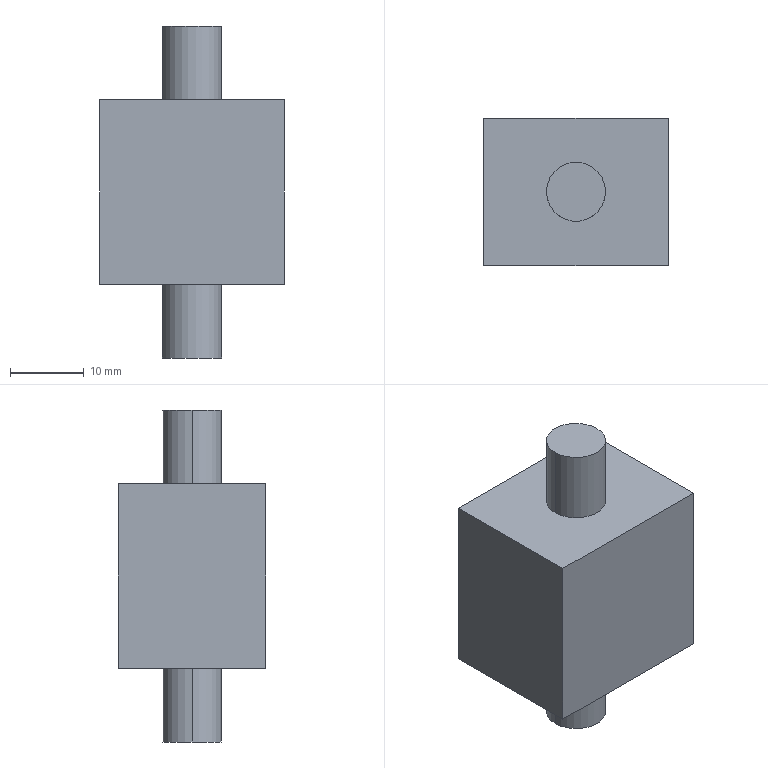Part | SolidWorks | features Extrusion 1, ICE 1, MirrorPattern 1 | 1 solid | 12 faces | box 25 x 20 x 45 mm | volume 13505 mm3 | plane 8 | cylinder 4 | commonest cylinder face diameters 8 x4
STEP:
#1=CARTESIAN_POINT('',(4.,10.,-22.5));
#2=VERTEX_POINT('',#1);
#3=CARTESIAN_POINT('',(-4.,10.,-22.5));
#4=VERTEX_POINT('',#3);
#5=CARTESIAN_POINT('',(0.,10.,-22.5));
#6=DIRECTION('',(0.,0.,1.));
#7=DIRECTION('',(1.,0.,0.));
#8=AXIS2_PLACEMENT_3D('',#5,#6,#7);
#9=CIRCLE('',#8,4.);
#10=EDGE_CURVE('',#2,#4,#9,.T.);
#11=ORIENTED_EDGE('',*,*,#10,.T.);
#12=CARTESIAN_POINT('',(-4.,10.,-12.5));
#13=VERTEX_POINT('',#12);
#14=CARTESIAN_POINT('',(-4.,10.,-22.5));
#15=DIRECTION('',(0.,0.,1.));
#16=VECTOR('',#15,1000.);
#17=LINE('',#14,#16);
#18=EDGE_CURVE('',#4,#13,#17,.T.);
#19=ORIENTED_EDGE('',*,*,#18,.T.);
#20=CARTESIAN_POINT('',(4.,10.,-12.5));
#21=VERTEX_POINT('',#20);
#22=CARTESIAN_POINT('',(0.,10.,-12.5));
#23=DIRECTION('',(0.,0.,1.));
#24=DIRECTION('',(1.,0.,0.));
#25=AXIS2_PLACEMENT_3D('',#22,#23,#24);
#26=CIRCLE('',#25,4.);
#27=EDGE_CURVE('',#21,#13,#26,.T.);
#28=ORIENTED_EDGE('',*,*,#27,.F.);
#29=CARTESIAN_POINT('',(4.,10.,-22.5));
#30=DIRECTION('',(0.,0.,1.));
#31=VECTOR('',#30,1000.);
#32=LINE('',#29,#31);
#33=EDGE_CURVE('',#2,#21,#32,.T.);
#34=ORIENTED_EDGE('',*,*,#33,.F.);
#35=EDGE_LOOP('',(#11,#19,#28,#34));
#36=FACE_OUTER_BOUND('',#35,.T.);
#37=CARTESIAN_POINT('',(0.,10.,-22.5));
#38=DIRECTION('',(0.,0.,1.));
#39=DIRECTION('',(1.,0.,0.));
#40=AXIS2_PLACEMENT_3D('',#37,#38,#39);
#41=CYLINDRICAL_SURFACE('',#40,4.);
#42=ADVANCED_FACE('',(#36),#41,.T.);
#43=CARTESIAN_POINT('',(4.,10.,22.5));
#44=VERTEX_POINT('',#43);
#45=CARTESIAN_POINT('',(-4.,10.,22.5));
#46=VERTEX_POINT('',#45);
#47=CARTESIAN_POINT('',(0.,10.,22.5));
#48=DIRECTION('',(0.,0.,1.));
#49=DIRECTION('',(1.,0.,0.));
#50=AXIS2_PLACEMENT_3D('',#47,#48,#49);
#51=CIRCLE('',#50,4.);
#52=EDGE_CURVE('',#44,#46,#51,.T.);
#53=ORIENTED_EDGE('',*,*,#52,.F.);
#54=CARTESIAN_POINT('',(4.,10.,12.5));
#55=VERTEX_POINT('',#54);
#56=CARTESIAN_POINT('',(4.,10.,22.5));
#57=DIRECTION('',(0.,0.,-1.));
#58=VECTOR('',#57,1000.);
#59=LINE('',#56,#58);
#60=EDGE_CURVE('',#44,#55,#59,.T.);
#61=ORIENTED_EDGE('',*,*,#60,.T.);
#62=CARTESIAN_POINT('',(-4.,10.,12.5));
#63=VERTEX_POINT('',#62);
#64=CARTESIAN_POINT('',(0.,10.,12.5));
#65=DIRECTION('',(0.,0.,1.));
#66=DIRECTION('',(1.,0.,0.));
#67=AXIS2_PLACEMENT_3D('',#64,#65,#66);
#68=CIRCLE('',#67,4.);
#69=EDGE_CURVE('',#55,#63,#68,.T.);
#70=ORIENTED_EDGE('',*,*,#69,.T.);
#71=CARTESIAN_POINT('',(-4.,10.,22.5));
#72=DIRECTION('',(0.,0.,-1.));
#73=VECTOR('',#72,1000.);
#74=LINE('',#71,#73);
#75=EDGE_CURVE('',#46,#63,#74,.T.);
#76=ORIENTED_EDGE('',*,*,#75,.F.);
#77=EDGE_LOOP('',(#53,#61,#70,#76));
#78=FACE_OUTER_BOUND('',#77,.T.);
#79=CARTESIAN_POINT('',(0.,10.,22.5));
#80=DIRECTION('',(0.,0.,-1.));
#81=DIRECTION('',(-1.,0.,0.));
#82=AXIS2_PLACEMENT_3D('',#79,#80,#81);
#83=CYLINDRICAL_SURFACE('',#82,4.);
#84=ADVANCED_FACE('',(#78),#83,.T.);
#85=CARTESIAN_POINT('',(12.5,0.,12.5));
#86=VERTEX_POINT('',#85);
#87=CARTESIAN_POINT('',(12.5,0.,-12.5));
#88=VERTEX_POINT('',#87);
#89=CARTESIAN_POINT('',(12.5,0.,12.5));
#90=DIRECTION('',(0.,0.,-1.));
#91=VECTOR('',#90,1000.);
#92=LINE('',#89,#91);
#93=EDGE_CURVE('',#86,#88,#92,.T.);
#94=ORIENTED_EDGE('',*,*,#93,.T.);
#95=CARTESIAN_POINT('',(12.5,20.,-12.5));
#96=VERTEX_POINT('',#95);
#97=CARTESIAN_POINT('',(12.5,20.,-12.5));
#98=DIRECTION('',(0.,-1.,0.));
#99=VECTOR('',#98,1000.);
#100=LINE('',#97,#99);
#101=EDGE_CURVE('',#96,#88,#100,.T.);
#102=ORIENTED_EDGE('',*,*,#101,.F.);
#103=CARTESIAN_POINT('',(12.5,20.,12.5));
#104=VERTEX_POINT('',#103);
#105=CARTESIAN_POINT('',(12.5,20.,12.5));
#106=DIRECTION('',(0.,0.,-1.));
#107=VECTOR('',#106,1000.);
#108=LINE('',#105,#107);
#109=EDGE_CURVE('',#104,#96,#108,.T.);
#110=ORIENTED_EDGE('',*,*,#109,.F.);
#111=CARTESIAN_POINT('',(12.5,20.,12.5));
#112=DIRECTION('',(0.,-1.,0.));
#113=VECTOR('',#112,1000.);
#114=LINE('',#111,#113);
#115=EDGE_CURVE('',#104,#86,#114,.T.);
#116=ORIENTED_EDGE('',*,*,#115,.T.);
#117=EDGE_LOOP('',(#94,#102,#110,#116));
#118=FACE_OUTER_BOUND('',#117,.T.);
#119=CARTESIAN_POINT('',(12.5,20.,12.5));
#120=DIRECTION('',(-1.,0.,0.));
#121=DIRECTION('',(0.,0.,1.));
#122=AXIS2_PLACEMENT_3D('',#119,#120,#121);
#123=PLANE('',#122);
#124=ADVANCED_FACE('',(#118),#123,.F.);
#125=ORIENTED_EDGE('',*,*,#27,.T.);
#126=CARTESIAN_POINT('',(0.,10.,-12.5));
#127=DIRECTION('',(0.,0.,1.));
#128=DIRECTION('',(1.,0.,0.));
#129=AXIS2_PLACEMENT_3D('',#126,#127,#128);
#130=CIRCLE('',#129,4.);
#131=EDGE_CURVE('',#13,#21,#130,.T.);
#132=ORIENTED_EDGE('',*,*,#131,.T.);
#133=EDGE_LOOP('',(#125,#132));
#134=FACE_BOUND('',#133,.T.);
#135=CARTESIAN_POINT('',(-12.5,0.,-12.5));
#136=VERTEX_POINT('',#135);
#137=CARTESIAN_POINT('',(-12.5,0.,-12.5));
#138=DIRECTION('',(-1.,0.,0.));
#139=VECTOR('',#138,1000.);
#140=LINE('',#137,#139);
#141=EDGE_CURVE('',#88,#136,#140,.T.);
#142=ORIENTED_EDGE('',*,*,#141,.T.);
#143=CARTESIAN_POINT('',(-12.5,20.,-12.5));
#144=VERTEX_POINT('',#143);
#145=CARTESIAN_POINT('',(-12.5,20.,-12.5));
#146=DIRECTION('',(0.,-1.,0.));
#147=VECTOR('',#146,1000.);
#148=LINE('',#145,#147);
#149=EDGE_CURVE('',#144,#136,#148,.T.);
#150=ORIENTED_EDGE('',*,*,#149,.F.);
#151=CARTESIAN_POINT('',(-12.5,20.,-12.5));
#152=DIRECTION('',(-1.,0.,0.));
#153=VECTOR('',#152,1000.);
#154=LINE('',#151,#153);
#155=EDGE_CURVE('',#96,#144,#154,.T.);
#156=ORIENTED_EDGE('',*,*,#155,.F.);
#157=ORIENTED_EDGE('',*,*,#101,.T.);
#158=EDGE_LOOP('',(#142,#150,#156,#157));
#159=FACE_OUTER_BOUND('',#158,.T.);
#160=CARTESIAN_POINT('',(-12.5,20.,-12.5));
#161=DIRECTION('',(0.,0.,1.));
#162=DIRECTION('',(1.,0.,0.));
#163=AXIS2_PLACEMENT_3D('',#160,#161,#162);
#164=PLANE('',#163);
#165=ADVANCED_FACE('',(#134,#159),#164,.F.);
#166=CARTESIAN_POINT('',(-12.5,0.,12.5));
#167=VERTEX_POINT('',#166);
#168=CARTESIAN_POINT('',(-12.5,0.,12.5));
#169=DIRECTION('',(0.,0.,1.));
#170=VECTOR('',#169,1000.);
#171=LINE('',#168,#170);
#172=EDGE_CURVE('',#136,#167,#171,.T.);
#173=ORIENTED_EDGE('',*,*,#172,.T.);
#174=CARTESIAN_POINT('',(-12.5,20.,12.5));
#175=VERTEX_POINT('',#174);
#176=CARTESIAN_POINT('',(-12.5,20.,12.5));
#177=DIRECTION('',(0.,-1.,0.));
#178=VECTOR('',#177,1000.);
#179=LINE('',#176,#178);
#180=EDGE_CURVE('',#175,#167,#179,.T.);
#181=ORIENTED_EDGE('',*,*,#180,.F.);
#182=CARTESIAN_POINT('',(-12.5,20.,12.5));
#183=DIRECTION('',(0.,0.,1.));
#184=VECTOR('',#183,1000.);
#185=LINE('',#182,#184);
#186=EDGE_CURVE('',#144,#175,#185,.T.);
#187=ORIENTED_EDGE('',*,*,#186,.F.);
#188=ORIENTED_EDGE('',*,*,#149,.T.);
#189=EDGE_LOOP('',(#173,#181,#187,#188));
#190=FACE_OUTER_BOUND('',#189,.T.);
#191=CARTESIAN_POINT('',(-12.5,20.,12.5));
#192=DIRECTION('',(1.,0.,0.));
#193=DIRECTION('',(0.,0.,-1.));
#194=AXIS2_PLACEMENT_3D('',#191,#192,#193);
#195=PLANE('',#194);
#196=ADVANCED_FACE('',(#190),#195,.F.);
#197=CARTESIAN_POINT('',(0.,10.,12.5));
#198=DIRECTION('',(0.,0.,1.));
#199=DIRECTION('',(1.,0.,0.));
#200=AXIS2_PLACEMENT_3D('',#197,#198,#199);
#201=CIRCLE('',#200,4.);
#202=EDGE_CURVE('',#63,#55,#201,.T.);
#203=ORIENTED_EDGE('',*,*,#202,.F.);
#204=ORIENTED_EDGE('',*,*,#69,.F.);
#205=EDGE_LOOP('',(#203,#204));
#206=FACE_BOUND('',#205,.T.);
#207=CARTESIAN_POINT('',(-12.5,0.,12.5));
#208=DIRECTION('',(1.,0.,0.));
#209=VECTOR('',#208,1000.);
#210=LINE('',#207,#209);
#211=EDGE_CURVE('',#167,#86,#210,.T.);
#212=ORIENTED_EDGE('',*,*,#211,.T.);
#213=ORIENTED_EDGE('',*,*,#115,.F.);
#214=CARTESIAN_POINT('',(-12.5,20.,12.5));
#215=DIRECTION('',(1.,0.,0.));
#216=VECTOR('',#215,1000.);
#217=LINE('',#214,#216);
#218=EDGE_CURVE('',#175,#104,#217,.T.);
#219=ORIENTED_EDGE('',*,*,#218,.F.);
#220=ORIENTED_EDGE('',*,*,#180,.T.);
#221=EDGE_LOOP('',(#212,#213,#219,#220));
#222=FACE_OUTER_BOUND('',#221,.T.);
#223=CARTESIAN_POINT('',(-12.5,20.,12.5));
#224=DIRECTION('',(0.,0.,-1.));
#225=DIRECTION('',(-1.,0.,0.));
#226=AXIS2_PLACEMENT_3D('',#223,#224,#225);
#227=PLANE('',#226);
#228=ADVANCED_FACE('',(#206,#222),#227,.F.);
#229=ORIENTED_EDGE('',*,*,#109,.T.);
#230=ORIENTED_EDGE('',*,*,#155,.T.);
#231=ORIENTED_EDGE('',*,*,#186,.T.);
#232=ORIENTED_EDGE('',*,*,#218,.T.);
#233=EDGE_LOOP('',(#229,#230,#231,#232));
#234=FACE_OUTER_BOUND('',#233,.T.);
#235=CARTESIAN_POINT('',(0.,20.,0.));
#236=DIRECTION('',(0.,-1.,0.));
#237=DIRECTION('',(0.,0.,-1.));
#238=AXIS2_PLACEMENT_3D('',#235,#236,#237);
#239=PLANE('',#238);
#240=ADVANCED_FACE('',(#234),#239,.F.);
#241=ORIENTED_EDGE('',*,*,#93,.F.);
#242=ORIENTED_EDGE('',*,*,#211,.F.);
#243=ORIENTED_EDGE('',*,*,#172,.F.);
#244=ORIENTED_EDGE('',*,*,#141,.F.);
#245=EDGE_LOOP('',(#241,#242,#243,#244));
#246=FACE_OUTER_BOUND('',#245,.T.);
#247=CARTESIAN_POINT('',(0.,0.,0.));
#248=DIRECTION('',(0.,-1.,0.));
#249=DIRECTION('',(0.,0.,-1.));
#250=AXIS2_PLACEMENT_3D('',#247,#248,#249);
#251=PLANE('',#250);
#252=ADVANCED_FACE('',(#246),#251,.T.);
#253=ORIENTED_EDGE('',*,*,#60,.F.);
#254=CARTESIAN_POINT('',(0.,10.,22.5));
#255=DIRECTION('',(0.,0.,1.));
#256=DIRECTION('',(1.,0.,0.));
#257=AXIS2_PLACEMENT_3D('',#254,#255,#256);
#258=CIRCLE('',#257,4.);
#259=EDGE_CURVE('',#46,#44,#258,.T.);
#260=ORIENTED_EDGE('',*,*,#259,.F.);
#261=ORIENTED_EDGE('',*,*,#75,.T.);
#262=ORIENTED_EDGE('',*,*,#202,.T.);
#263=EDGE_LOOP('',(#253,#260,#261,#262));
#264=FACE_OUTER_BOUND('',#263,.T.);
#265=CARTESIAN_POINT('',(0.,10.,22.5));
#266=DIRECTION('',(0.,0.,-1.));
#267=DIRECTION('',(-1.,0.,0.));
#268=AXIS2_PLACEMENT_3D('',#265,#266,#267);
#269=CYLINDRICAL_SURFACE('',#268,4.);
#270=ADVANCED_FACE('',(#264),#269,.T.);
#271=ORIENTED_EDGE('',*,*,#259,.T.);
#272=ORIENTED_EDGE('',*,*,#52,.T.);
#273=EDGE_LOOP('',(#271,#272));
#274=FACE_OUTER_BOUND('',#273,.T.);
#275=CARTESIAN_POINT('',(0.,10.,22.5));
#276=DIRECTION('',(0.,0.,1.));
#277=DIRECTION('',(1.,0.,0.));
#278=AXIS2_PLACEMENT_3D('',#275,#276,#277);
#279=PLANE('',#278);
#280=ADVANCED_FACE('',(#274),#279,.T.);
#281=ORIENTED_EDGE('',*,*,#18,.F.);
#282=CARTESIAN_POINT('',(0.,10.,-22.5));
#283=DIRECTION('',(0.,0.,1.));
#284=DIRECTION('',(1.,0.,0.));
#285=AXIS2_PLACEMENT_3D('',#282,#283,#284);
#286=CIRCLE('',#285,4.);
#287=EDGE_CURVE('',#4,#2,#286,.T.);
#288=ORIENTED_EDGE('',*,*,#287,.T.);
#289=ORIENTED_EDGE('',*,*,#33,.T.);
#290=ORIENTED_EDGE('',*,*,#131,.F.);
#291=EDGE_LOOP('',(#281,#288,#289,#290));
#292=FACE_OUTER_BOUND('',#291,.T.);
#293=CARTESIAN_POINT('',(0.,10.,-22.5));
#294=DIRECTION('',(0.,0.,1.));
#295=DIRECTION('',(1.,0.,0.));
#296=AXIS2_PLACEMENT_3D('',#293,#294,#295);
#297=CYLINDRICAL_SURFACE('',#296,4.);
#298=ADVANCED_FACE('',(#292),#297,.T.);
#299=ORIENTED_EDGE('',*,*,#10,.F.);
#300=ORIENTED_EDGE('',*,*,#287,.F.);
#301=EDGE_LOOP('',(#299,#300));
#302=FACE_OUTER_BOUND('',#301,.T.);
#303=CARTESIAN_POINT('',(0.,10.,-22.5));
#304=DIRECTION('',(0.,0.,-1.));
#305=DIRECTION('',(1.,0.,0.));
#306=AXIS2_PLACEMENT_3D('',#303,#304,#305);
#307=PLANE('',#306);
#308=ADVANCED_FACE('',(#302),#307,.T.);
#309=CLOSED_SHELL('',(#42,#84,#124,#165,#196,#228,#240,#252,#270,#280,#298,#308));
#310=MANIFOLD_SOLID_BREP('',#309);
#311=CARTESIAN_POINT('',(0.,0.,0.));
#312=DIRECTION('',(0.,0.,1.));
#313=DIRECTION('',(1.,0.,0.));
#314=AXIS2_PLACEMENT_3D('',#311,#312,#313);
#315=(LENGTH_UNIT()NAMED_UNIT(*)SI_UNIT(.MILLI.,.METRE.));
#316=UNCERTAINTY_MEASURE_WITH_UNIT(LENGTH_MEASURE(0.00001),#315,'','');
#317=(NAMED_UNIT(*)PLANE_ANGLE_UNIT()SI_UNIT($,.RADIAN.));
#318=(NAMED_UNIT(*)SI_UNIT($,.STERADIAN.)SOLID_ANGLE_UNIT());
#319=(GEOMETRIC_REPRESENTATION_CONTEXT(3)GLOBAL_UNCERTAINTY_ASSIGNED_CONTEXT((#316))GLOBAL_UNIT_ASSIGNED_CONTEXT((#315,#317,#318))REPRESENTATION_CONTEXT('',''));
#320=ADVANCED_BREP_SHAPE_REPRESENTATION('',(#310,#314),#319);